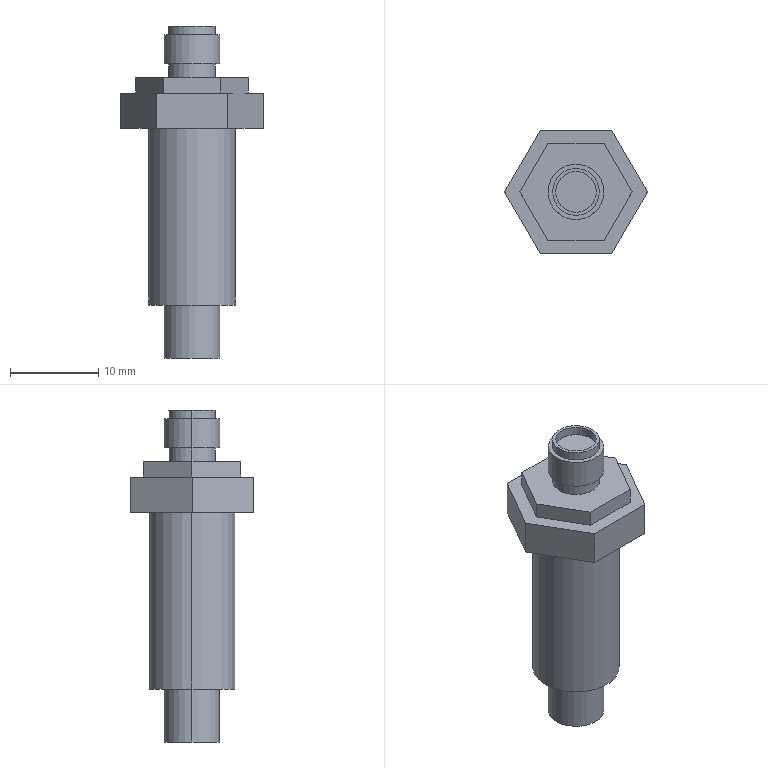Part | SolidWorks | features ICE 5, Extrusion 1 | 1 solid | 40 faces | box 16.166 x 14 x 37.6 mm | volume 2584 mm3 | plane 24 | cylinder 16 | commonest cylinder face diameters 4.6 x4 5.3 x4 6.3 x4 4.5 x2 9.8 x2
STEP:
#1=CARTESIAN_POINT('',(2.25,0.,-26.));
#2=VERTEX_POINT('',#1);
#3=CARTESIAN_POINT('',(-2.25,0.,-26.));
#4=VERTEX_POINT('',#3);
#5=CARTESIAN_POINT('',(0.,0.,-26.));
#6=DIRECTION('',(0.,0.,-1.));
#7=DIRECTION('',(-1.,0.,0.));
#8=AXIS2_PLACEMENT_3D('',#5,#6,#7);
#9=CIRCLE('',#8,2.25);
#10=EDGE_CURVE('',#2,#4,#9,.T.);
#11=ORIENTED_EDGE('',*,*,#10,.T.);
#12=CARTESIAN_POINT('',(-2.25,0.,-20.));
#13=VERTEX_POINT('',#12);
#14=CARTESIAN_POINT('',(-2.25,0.,-26.));
#15=DIRECTION('',(0.,0.,1.));
#16=VECTOR('',#15,1000.);
#17=LINE('',#14,#16);
#18=EDGE_CURVE('',#4,#13,#17,.T.);
#19=ORIENTED_EDGE('',*,*,#18,.T.);
#20=CARTESIAN_POINT('',(2.25,0.,-20.));
#21=VERTEX_POINT('',#20);
#22=CARTESIAN_POINT('',(0.,0.,-20.));
#23=DIRECTION('',(0.,0.,1.));
#24=DIRECTION('',(-1.,0.,0.));
#25=AXIS2_PLACEMENT_3D('',#22,#23,#24);
#26=CIRCLE('',#25,2.25);
#27=EDGE_CURVE('',#13,#21,#26,.T.);
#28=ORIENTED_EDGE('',*,*,#27,.T.);
#29=CARTESIAN_POINT('',(2.25,0.,-26.));
#30=DIRECTION('',(0.,0.,1.));
#31=VECTOR('',#30,1000.);
#32=LINE('',#29,#31);
#33=EDGE_CURVE('',#2,#21,#32,.T.);
#34=ORIENTED_EDGE('',*,*,#33,.F.);
#35=EDGE_LOOP('',(#11,#19,#28,#34));
#36=FACE_OUTER_BOUND('',#35,.T.);
#37=CARTESIAN_POINT('',(0.,0.,-26.));
#38=DIRECTION('',(0.,0.,1.));
#39=DIRECTION('',(1.,0.,0.));
#40=AXIS2_PLACEMENT_3D('',#37,#38,#39);
#41=CYLINDRICAL_SURFACE('',#40,2.25);
#42=ADVANCED_FACE('',(#36),#41,.F.);
#43=CARTESIAN_POINT('',(-3.15,0.,-26.));
#44=VERTEX_POINT('',#43);
#45=CARTESIAN_POINT('',(3.15,0.,-26.));
#46=VERTEX_POINT('',#45);
#47=CARTESIAN_POINT('',(0.,0.,-26.));
#48=DIRECTION('',(0.,0.,-1.));
#49=DIRECTION('',(-1.,0.,0.));
#50=AXIS2_PLACEMENT_3D('',#47,#48,#49);
#51=CIRCLE('',#50,3.15);
#52=EDGE_CURVE('',#44,#46,#51,.T.);
#53=ORIENTED_EDGE('',*,*,#52,.F.);
#54=CARTESIAN_POINT('',(-3.15,0.,-20.));
#55=VERTEX_POINT('',#54);
#56=CARTESIAN_POINT('',(-3.15,0.,-26.));
#57=DIRECTION('',(0.,0.,1.));
#58=VECTOR('',#57,1000.);
#59=LINE('',#56,#58);
#60=EDGE_CURVE('',#44,#55,#59,.T.);
#61=ORIENTED_EDGE('',*,*,#60,.T.);
#62=CARTESIAN_POINT('',(3.15,0.,-20.));
#63=VERTEX_POINT('',#62);
#64=CARTESIAN_POINT('',(0.,0.,-20.));
#65=DIRECTION('',(0.,0.,-1.));
#66=DIRECTION('',(-1.,0.,0.));
#67=AXIS2_PLACEMENT_3D('',#64,#65,#66);
#68=CIRCLE('',#67,3.15);
#69=EDGE_CURVE('',#55,#63,#68,.T.);
#70=ORIENTED_EDGE('',*,*,#69,.T.);
#71=CARTESIAN_POINT('',(3.15,0.,-26.));
#72=DIRECTION('',(0.,0.,1.));
#73=VECTOR('',#72,1000.);
#74=LINE('',#71,#73);
#75=EDGE_CURVE('',#46,#63,#74,.T.);
#76=ORIENTED_EDGE('',*,*,#75,.F.);
#77=EDGE_LOOP('',(#53,#61,#70,#76));
#78=FACE_OUTER_BOUND('',#77,.T.);
#79=CARTESIAN_POINT('',(0.,0.,-26.));
#80=DIRECTION('',(0.,0.,1.));
#81=DIRECTION('',(1.,0.,0.));
#82=AXIS2_PLACEMENT_3D('',#79,#80,#81);
#83=CYLINDRICAL_SURFACE('',#82,3.15);
#84=ADVANCED_FACE('',(#78),#83,.T.);
#85=CARTESIAN_POINT('',(-4.9,0.,-20.));
#86=VERTEX_POINT('',#85);
#87=CARTESIAN_POINT('',(4.9,0.,-20.));
#88=VERTEX_POINT('',#87);
#89=CARTESIAN_POINT('',(0.,0.,-20.));
#90=DIRECTION('',(0.,0.,-1.));
#91=DIRECTION('',(-1.,0.,0.));
#92=AXIS2_PLACEMENT_3D('',#89,#90,#91);
#93=CIRCLE('',#92,4.9);
#94=EDGE_CURVE('',#86,#88,#93,.T.);
#95=ORIENTED_EDGE('',*,*,#94,.F.);
#96=CARTESIAN_POINT('',(-4.9,0.,0.));
#97=VERTEX_POINT('',#96);
#98=CARTESIAN_POINT('',(-4.9,0.,-20.));
#99=DIRECTION('',(0.,0.,1.));
#100=VECTOR('',#99,1000.);
#101=LINE('',#98,#100);
#102=EDGE_CURVE('',#86,#97,#101,.T.);
#103=ORIENTED_EDGE('',*,*,#102,.T.);
#104=CARTESIAN_POINT('',(4.9,0.,0.));
#105=VERTEX_POINT('',#104);
#106=CARTESIAN_POINT('',(0.,0.,0.));
#107=DIRECTION('',(0.,0.,-1.));
#108=DIRECTION('',(-1.,0.,0.));
#109=AXIS2_PLACEMENT_3D('',#106,#107,#108);
#110=CIRCLE('',#109,4.9);
#111=EDGE_CURVE('',#97,#105,#110,.T.);
#112=ORIENTED_EDGE('',*,*,#111,.T.);
#113=CARTESIAN_POINT('',(4.9,0.,-20.));
#114=DIRECTION('',(0.,0.,1.));
#115=VECTOR('',#114,1000.);
#116=LINE('',#113,#115);
#117=EDGE_CURVE('',#88,#105,#116,.T.);
#118=ORIENTED_EDGE('',*,*,#117,.F.);
#119=EDGE_LOOP('',(#95,#103,#112,#118));
#120=FACE_OUTER_BOUND('',#119,.T.);
#121=CARTESIAN_POINT('',(0.,0.,-20.));
#122=DIRECTION('',(0.,0.,1.));
#123=DIRECTION('',(1.,0.,0.));
#124=AXIS2_PLACEMENT_3D('',#121,#122,#123);
#125=CYLINDRICAL_SURFACE('',#124,4.9);
#126=ADVANCED_FACE('',(#120),#125,.T.);
#127=CARTESIAN_POINT('',(-2.3,0.,11.6));
#128=VERTEX_POINT('',#127);
#129=CARTESIAN_POINT('',(2.3,0.,11.6));
#130=VERTEX_POINT('',#129);
#131=CARTESIAN_POINT('',(0.,0.,11.6));
#132=DIRECTION('',(0.,0.,1.));
#133=DIRECTION('',(1.,0.,0.));
#134=AXIS2_PLACEMENT_3D('',#131,#132,#133);
#135=CIRCLE('',#134,2.3);
#136=EDGE_CURVE('',#128,#130,#135,.T.);
#137=ORIENTED_EDGE('',*,*,#136,.T.);
#138=CARTESIAN_POINT('',(2.3,0.,10.6));
#139=VERTEX_POINT('',#138);
#140=CARTESIAN_POINT('',(2.3,0.,11.6));
#141=DIRECTION('',(0.,0.,-1.));
#142=VECTOR('',#141,1000.);
#143=LINE('',#140,#142);
#144=EDGE_CURVE('',#130,#139,#143,.T.);
#145=ORIENTED_EDGE('',*,*,#144,.T.);
#146=CARTESIAN_POINT('',(-2.3,0.,10.6));
#147=VERTEX_POINT('',#146);
#148=CARTESIAN_POINT('',(0.,0.,10.6));
#149=DIRECTION('',(0.,0.,1.));
#150=DIRECTION('',(1.,0.,0.));
#151=AXIS2_PLACEMENT_3D('',#148,#149,#150);
#152=CIRCLE('',#151,2.3);
#153=EDGE_CURVE('',#147,#139,#152,.T.);
#154=ORIENTED_EDGE('',*,*,#153,.F.);
#155=CARTESIAN_POINT('',(-2.3,0.,11.6));
#156=DIRECTION('',(0.,0.,-1.));
#157=VECTOR('',#156,1000.);
#158=LINE('',#155,#157);
#159=EDGE_CURVE('',#128,#147,#158,.T.);
#160=ORIENTED_EDGE('',*,*,#159,.F.);
#161=EDGE_LOOP('',(#137,#145,#154,#160));
#162=FACE_OUTER_BOUND('',#161,.T.);
#163=CARTESIAN_POINT('',(0.,0.,11.6));
#164=DIRECTION('',(0.,0.,-1.));
#165=DIRECTION('',(-1.,0.,0.));
#166=AXIS2_PLACEMENT_3D('',#163,#164,#165);
#167=CYLINDRICAL_SURFACE('',#166,2.3);
#168=ADVANCED_FACE('',(#162),#167,.F.);
#169=CARTESIAN_POINT('',(2.65,0.,11.6));
#170=VERTEX_POINT('',#169);
#171=CARTESIAN_POINT('',(-2.65,0.,11.6));
#172=VERTEX_POINT('',#171);
#173=CARTESIAN_POINT('',(0.,0.,11.6));
#174=DIRECTION('',(0.,0.,1.));
#175=DIRECTION('',(1.,0.,0.));
#176=AXIS2_PLACEMENT_3D('',#173,#174,#175);
#177=CIRCLE('',#176,2.65);
#178=EDGE_CURVE('',#170,#172,#177,.T.);
#179=ORIENTED_EDGE('',*,*,#178,.F.);
#180=CARTESIAN_POINT('',(2.65,0.,10.6));
#181=VERTEX_POINT('',#180);
#182=CARTESIAN_POINT('',(2.65,0.,11.6));
#183=DIRECTION('',(0.,0.,-1.));
#184=VECTOR('',#183,1000.);
#185=LINE('',#182,#184);
#186=EDGE_CURVE('',#170,#181,#185,.T.);
#187=ORIENTED_EDGE('',*,*,#186,.T.);
#188=CARTESIAN_POINT('',(-2.65,0.,10.6));
#189=VERTEX_POINT('',#188);
#190=CARTESIAN_POINT('',(0.,0.,10.6));
#191=DIRECTION('',(0.,0.,1.));
#192=DIRECTION('',(1.,0.,0.));
#193=AXIS2_PLACEMENT_3D('',#190,#191,#192);
#194=CIRCLE('',#193,2.65);
#195=EDGE_CURVE('',#181,#189,#194,.T.);
#196=ORIENTED_EDGE('',*,*,#195,.T.);
#197=CARTESIAN_POINT('',(-2.65,0.,11.6));
#198=DIRECTION('',(0.,0.,-1.));
#199=VECTOR('',#198,1000.);
#200=LINE('',#197,#199);
#201=EDGE_CURVE('',#172,#189,#200,.T.);
#202=ORIENTED_EDGE('',*,*,#201,.F.);
#203=EDGE_LOOP('',(#179,#187,#196,#202));
#204=FACE_OUTER_BOUND('',#203,.T.);
#205=CARTESIAN_POINT('',(0.,0.,11.6));
#206=DIRECTION('',(0.,0.,-1.));
#207=DIRECTION('',(-1.,0.,0.));
#208=AXIS2_PLACEMENT_3D('',#205,#206,#207);
#209=CYLINDRICAL_SURFACE('',#208,2.65);
#210=ADVANCED_FACE('',(#204),#209,.T.);
#211=CARTESIAN_POINT('',(3.15,0.,7.3));
#212=VERTEX_POINT('',#211);
#213=CARTESIAN_POINT('',(-3.15,0.,7.3));
#214=VERTEX_POINT('',#213);
#215=CARTESIAN_POINT('',(0.,0.,7.3));
#216=DIRECTION('',(0.,0.,1.));
#217=DIRECTION('',(1.,0.,0.));
#218=AXIS2_PLACEMENT_3D('',#215,#216,#217);
#219=CIRCLE('',#218,3.15);
#220=EDGE_CURVE('',#212,#214,#219,.T.);
#221=ORIENTED_EDGE('',*,*,#220,.T.);
#222=CARTESIAN_POINT('',(-3.15,0.,10.6));
#223=VERTEX_POINT('',#222);
#224=CARTESIAN_POINT('',(-3.15,0.,7.3));
#225=DIRECTION('',(0.,0.,1.));
#226=VECTOR('',#225,1000.);
#227=LINE('',#224,#226);
#228=EDGE_CURVE('',#214,#223,#227,.T.);
#229=ORIENTED_EDGE('',*,*,#228,.T.);
#230=CARTESIAN_POINT('',(3.15,0.,10.6));
#231=VERTEX_POINT('',#230);
#232=CARTESIAN_POINT('',(0.,0.,10.6));
#233=DIRECTION('',(0.,0.,1.));
#234=DIRECTION('',(1.,0.,0.));
#235=AXIS2_PLACEMENT_3D('',#232,#233,#234);
#236=CIRCLE('',#235,3.15);
#237=EDGE_CURVE('',#231,#223,#236,.T.);
#238=ORIENTED_EDGE('',*,*,#237,.F.);
#239=CARTESIAN_POINT('',(3.15,0.,7.3));
#240=DIRECTION('',(0.,0.,1.));
#241=VECTOR('',#240,1000.);
#242=LINE('',#239,#241);
#243=EDGE_CURVE('',#212,#231,#242,.T.);
#244=ORIENTED_EDGE('',*,*,#243,.F.);
#245=EDGE_LOOP('',(#221,#229,#238,#244));
#246=FACE_OUTER_BOUND('',#245,.T.);
#247=CARTESIAN_POINT('',(0.,0.,7.3));
#248=DIRECTION('',(0.,0.,1.));
#249=DIRECTION('',(1.,0.,0.));
#250=AXIS2_PLACEMENT_3D('',#247,#248,#249);
#251=CYLINDRICAL_SURFACE('',#250,3.15);
#252=ADVANCED_FACE('',(#246),#251,.T.);
#253=CARTESIAN_POINT('',(2.65,0.,7.3));
#254=VERTEX_POINT('',#253);
#255=CARTESIAN_POINT('',(-2.65,0.,7.3));
#256=VERTEX_POINT('',#255);
#257=CARTESIAN_POINT('',(0.,0.,7.3));
#258=DIRECTION('',(0.,0.,1.));
#259=DIRECTION('',(1.,0.,0.));
#260=AXIS2_PLACEMENT_3D('',#257,#258,#259);
#261=CIRCLE('',#260,2.65);
#262=EDGE_CURVE('',#254,#256,#261,.T.);
#263=ORIENTED_EDGE('',*,*,#262,.F.);
#264=CARTESIAN_POINT('',(2.65,0.,5.8));
#265=VERTEX_POINT('',#264);
#266=CARTESIAN_POINT('',(2.65,0.,11.6));
#267=DIRECTION('',(0.,0.,-1.));
#268=VECTOR('',#267,1000.);
#269=LINE('',#266,#268);
#270=EDGE_CURVE('',#254,#265,#269,.T.);
#271=ORIENTED_EDGE('',*,*,#270,.T.);
#272=CARTESIAN_POINT('',(-2.65,0.,5.8));
#273=VERTEX_POINT('',#272);
#274=CARTESIAN_POINT('',(0.,0.,5.8));
#275=DIRECTION('',(0.,0.,1.));
#276=DIRECTION('',(1.,0.,0.));
#277=AXIS2_PLACEMENT_3D('',#274,#275,#276);
#278=CIRCLE('',#277,2.65);
#279=EDGE_CURVE('',#265,#273,#278,.T.);
#280=ORIENTED_EDGE('',*,*,#279,.T.);
#281=CARTESIAN_POINT('',(-2.65,0.,11.6));
#282=DIRECTION('',(0.,0.,-1.));
#283=VECTOR('',#282,1000.);
#284=LINE('',#281,#283);
#285=EDGE_CURVE('',#256,#273,#284,.T.);
#286=ORIENTED_EDGE('',*,*,#285,.F.);
#287=EDGE_LOOP('',(#263,#271,#280,#286));
#288=FACE_OUTER_BOUND('',#287,.T.);
#289=CARTESIAN_POINT('',(0.,0.,11.6));
#290=DIRECTION('',(0.,0.,-1.));
#291=DIRECTION('',(-1.,0.,0.));
#292=AXIS2_PLACEMENT_3D('',#289,#290,#291);
#293=CYLINDRICAL_SURFACE('',#292,2.65);
#294=ADVANCED_FACE('',(#288),#293,.T.);
#295=ORIENTED_EDGE('',*,*,#270,.F.);
#296=CARTESIAN_POINT('',(0.,0.,7.3));
#297=DIRECTION('',(0.,0.,1.));
#298=DIRECTION('',(1.,0.,0.));
#299=AXIS2_PLACEMENT_3D('',#296,#297,#298);
#300=CIRCLE('',#299,2.65);
#301=EDGE_CURVE('',#256,#254,#300,.T.);
#302=ORIENTED_EDGE('',*,*,#301,.F.);
#303=ORIENTED_EDGE('',*,*,#285,.T.);
#304=CARTESIAN_POINT('',(0.,0.,5.8));
#305=DIRECTION('',(0.,0.,1.));
#306=DIRECTION('',(1.,0.,0.));
#307=AXIS2_PLACEMENT_3D('',#304,#305,#306);
#308=CIRCLE('',#307,2.65);
#309=EDGE_CURVE('',#273,#265,#308,.T.);
#310=ORIENTED_EDGE('',*,*,#309,.T.);
#311=EDGE_LOOP('',(#295,#302,#303,#310));
#312=FACE_OUTER_BOUND('',#311,.T.);
#313=CARTESIAN_POINT('',(0.,0.,11.6));
#314=DIRECTION('',(0.,0.,-1.));
#315=DIRECTION('',(-1.,0.,0.));
#316=AXIS2_PLACEMENT_3D('',#313,#314,#315);
#317=CYLINDRICAL_SURFACE('',#316,2.65);
#318=ADVANCED_FACE('',(#312),#317,.T.);
#319=CARTESIAN_POINT('',(4.041,-7.,0.));
#320=VERTEX_POINT('',#319);
#321=CARTESIAN_POINT('',(8.083,0.,0.));
#322=VERTEX_POINT('',#321);
#323=CARTESIAN_POINT('',(4.041,-7.,0.));
#324=DIRECTION('',(0.5,0.866,0.));
#325=VECTOR('',#324,1000.);
#326=LINE('',#323,#325);
#327=EDGE_CURVE('',#320,#322,#326,.T.);
#328=ORIENTED_EDGE('',*,*,#327,.T.);
#329=CARTESIAN_POINT('',(8.083,0.,4.));
#330=VERTEX_POINT('',#329);
#331=CARTESIAN_POINT('',(8.083,0.,4.));
#332=DIRECTION('',(0.,0.,-1.));
#333=VECTOR('',#332,1000.);
#334=LINE('',#331,#333);
#335=EDGE_CURVE('',#330,#322,#334,.T.);
#336=ORIENTED_EDGE('',*,*,#335,.F.);
#337=CARTESIAN_POINT('',(4.041,-7.,4.));
#338=VERTEX_POINT('',#337);
#339=CARTESIAN_POINT('',(4.041,-7.,4.));
#340=DIRECTION('',(0.5,0.866,0.));
#341=VECTOR('',#340,1000.);
#342=LINE('',#339,#341);
#343=EDGE_CURVE('',#338,#330,#342,.T.);
#344=ORIENTED_EDGE('',*,*,#343,.F.);
#345=CARTESIAN_POINT('',(4.041,-7.,4.));
#346=DIRECTION('',(0.,0.,-1.));
#347=VECTOR('',#346,1000.);
#348=LINE('',#345,#347);
#349=EDGE_CURVE('',#338,#320,#348,.T.);
#350=ORIENTED_EDGE('',*,*,#349,.T.);
#351=EDGE_LOOP('',(#328,#336,#344,#350));
#352=FACE_OUTER_BOUND('',#351,.T.);
#353=CARTESIAN_POINT('',(4.041,-7.,4.));
#354=DIRECTION('',(-0.866,0.5,0.));
#355=DIRECTION('',(-0.5,-0.866,0.));
#356=AXIS2_PLACEMENT_3D('',#353,#354,#355);
#357=PLANE('',#356);
#358=ADVANCED_FACE('',(#352),#357,.F.);
#359=CARTESIAN_POINT('',(4.041,7.,0.));
#360=VERTEX_POINT('',#359);
#361=CARTESIAN_POINT('',(8.083,0.,0.));
#362=DIRECTION('',(-0.5,0.866,0.));
#363=VECTOR('',#362,1000.);
#364=LINE('',#361,#363);
#365=EDGE_CURVE('',#322,#360,#364,.T.);
#366=ORIENTED_EDGE('',*,*,#365,.T.);
#367=CARTESIAN_POINT('',(4.041,7.,4.));
#368=VERTEX_POINT('',#367);
#369=CARTESIAN_POINT('',(4.041,7.,4.));
#370=DIRECTION('',(0.,0.,-1.));
#371=VECTOR('',#370,1000.);
#372=LINE('',#369,#371);
#373=EDGE_CURVE('',#368,#360,#372,.T.);
#374=ORIENTED_EDGE('',*,*,#373,.F.);
#375=CARTESIAN_POINT('',(8.083,0.,4.));
#376=DIRECTION('',(-0.5,0.866,0.));
#377=VECTOR('',#376,1000.);
#378=LINE('',#375,#377);
#379=EDGE_CURVE('',#330,#368,#378,.T.);
#380=ORIENTED_EDGE('',*,*,#379,.F.);
#381=ORIENTED_EDGE('',*,*,#335,.T.);
#382=EDGE_LOOP('',(#366,#374,#380,#381));
#383=FACE_OUTER_BOUND('',#382,.T.);
#384=CARTESIAN_POINT('',(8.083,0.,4.));
#385=DIRECTION('',(-0.866,-0.5,0.));
#386=DIRECTION('',(0.5,-0.866,0.));
#387=AXIS2_PLACEMENT_3D('',#384,#385,#386);
#388=PLANE('',#387);
#389=ADVANCED_FACE('',(#383),#388,.F.);
#390=CARTESIAN_POINT('',(-4.041,7.,0.));
#391=VERTEX_POINT('',#390);
#392=CARTESIAN_POINT('',(4.041,7.,0.));
#393=DIRECTION('',(-1.,0.,0.));
#394=VECTOR('',#393,1000.);
#395=LINE('',#392,#394);
#396=EDGE_CURVE('',#360,#391,#395,.T.);
#397=ORIENTED_EDGE('',*,*,#396,.T.);
#398=CARTESIAN_POINT('',(-4.041,7.,4.));
#399=VERTEX_POINT('',#398);
#400=CARTESIAN_POINT('',(-4.041,7.,4.));
#401=DIRECTION('',(0.,0.,-1.));
#402=VECTOR('',#401,1000.);
#403=LINE('',#400,#402);
#404=EDGE_CURVE('',#399,#391,#403,.T.);
#405=ORIENTED_EDGE('',*,*,#404,.F.);
#406=CARTESIAN_POINT('',(4.041,7.,4.));
#407=DIRECTION('',(-1.,0.,0.));
#408=VECTOR('',#407,1000.);
#409=LINE('',#406,#408);
#410=EDGE_CURVE('',#368,#399,#409,.T.);
#411=ORIENTED_EDGE('',*,*,#410,.F.);
#412=ORIENTED_EDGE('',*,*,#373,.T.);
#413=EDGE_LOOP('',(#397,#405,#411,#412));
#414=FACE_OUTER_BOUND('',#413,.T.);
#415=CARTESIAN_POINT('',(4.041,7.,4.));
#416=DIRECTION('',(0.,-1.,0.));
#417=DIRECTION('',(1.,0.,0.));
#418=AXIS2_PLACEMENT_3D('',#415,#416,#417);
#419=PLANE('',#418);
#420=ADVANCED_FACE('',(#414),#419,.F.);
#421=CARTESIAN_POINT('',(-8.083,0.,0.));
#422=VERTEX_POINT('',#421);
#423=CARTESIAN_POINT('',(-4.041,7.,0.));
#424=DIRECTION('',(-0.5,-0.866,0.));
#425=VECTOR('',#424,1000.);
#426=LINE('',#423,#425);
#427=EDGE_CURVE('',#391,#422,#426,.T.);
#428=ORIENTED_EDGE('',*,*,#427,.T.);
#429=CARTESIAN_POINT('',(-8.083,0.,4.));
#430=VERTEX_POINT('',#429);
#431=CARTESIAN_POINT('',(-8.083,0.,4.));
#432=DIRECTION('',(0.,0.,-1.));
#433=VECTOR('',#432,1000.);
#434=LINE('',#431,#433);
#435=EDGE_CURVE('',#430,#422,#434,.T.);
#436=ORIENTED_EDGE('',*,*,#435,.F.);
#437=CARTESIAN_POINT('',(-4.041,7.,4.));
#438=DIRECTION('',(-0.5,-0.866,0.));
#439=VECTOR('',#438,1000.);
#440=LINE('',#437,#439);
#441=EDGE_CURVE('',#399,#430,#440,.T.);
#442=ORIENTED_EDGE('',*,*,#441,.F.);
#443=ORIENTED_EDGE('',*,*,#404,.T.);
#444=EDGE_LOOP('',(#428,#436,#442,#443));
#445=FACE_OUTER_BOUND('',#444,.T.);
#446=CARTESIAN_POINT('',(-4.041,7.,4.));
#447=DIRECTION('',(0.866,-0.5,0.));
#448=DIRECTION('',(0.5,0.866,0.));
#449=AXIS2_PLACEMENT_3D('',#446,#447,#448);
#450=PLANE('',#449);
#451=ADVANCED_FACE('',(#445),#450,.F.);
#452=CARTESIAN_POINT('',(-4.041,-7.,0.));
#453=VERTEX_POINT('',#452);
#454=CARTESIAN_POINT('',(-8.083,0.,0.));
#455=DIRECTION('',(0.5,-0.866,0.));
#456=VECTOR('',#455,1000.);
#457=LINE('',#454,#456);
#458=EDGE_CURVE('',#422,#453,#457,.T.);
#459=ORIENTED_EDGE('',*,*,#458,.T.);
#460=CARTESIAN_POINT('',(-4.041,-7.,4.));
#461=VERTEX_POINT('',#460);
#462=CARTESIAN_POINT('',(-4.041,-7.,4.));
#463=DIRECTION('',(0.,0.,-1.));
#464=VECTOR('',#463,1000.);
#465=LINE('',#462,#464);
#466=EDGE_CURVE('',#461,#453,#465,.T.);
#467=ORIENTED_EDGE('',*,*,#466,.F.);
#468=CARTESIAN_POINT('',(-8.083,0.,4.));
#469=DIRECTION('',(0.5,-0.866,0.));
#470=VECTOR('',#469,1000.);
#471=LINE('',#468,#470);
#472=EDGE_CURVE('',#430,#461,#471,.T.);
#473=ORIENTED_EDGE('',*,*,#472,.F.);
#474=ORIENTED_EDGE('',*,*,#435,.T.);
#475=EDGE_LOOP('',(#459,#467,#473,#474));
#476=FACE_OUTER_BOUND('',#475,.T.);
#477=CARTESIAN_POINT('',(-8.083,0.,4.));
#478=DIRECTION('',(0.866,0.5,0.));
#479=DIRECTION('',(-0.5,0.866,0.));
#480=AXIS2_PLACEMENT_3D('',#477,#478,#479);
#481=PLANE('',#480);
#482=ADVANCED_FACE('',(#476),#481,.F.);
#483=CARTESIAN_POINT('',(-4.041,-7.,0.));
#484=DIRECTION('',(1.,0.,0.));
#485=VECTOR('',#484,1000.);
#486=LINE('',#483,#485);
#487=EDGE_CURVE('',#453,#320,#486,.T.);
#488=ORIENTED_EDGE('',*,*,#487,.T.);
#489=ORIENTED_EDGE('',*,*,#349,.F.);
#490=CARTESIAN_POINT('',(-4.041,-7.,4.));
#491=DIRECTION('',(1.,0.,0.));
#492=VECTOR('',#491,1000.);
#493=LINE('',#490,#492);
#494=EDGE_CURVE('',#461,#338,#493,.T.);
#495=ORIENTED_EDGE('',*,*,#494,.F.);
#496=ORIENTED_EDGE('',*,*,#466,.T.);
#497=EDGE_LOOP('',(#488,#489,#495,#496));
#498=FACE_OUTER_BOUND('',#497,.T.);
#499=CARTESIAN_POINT('',(-4.041,-7.,4.));
#500=DIRECTION('',(0.,1.,0.));
#501=DIRECTION('',(-1.,0.,0.));
#502=AXIS2_PLACEMENT_3D('',#499,#500,#501);
#503=PLANE('',#502);
#504=ADVANCED_FACE('',(#498),#503,.F.);
#505=CARTESIAN_POINT('',(3.175,-5.5,4.));
#506=VERTEX_POINT('',#505);
#507=CARTESIAN_POINT('',(6.351,0.,4.));
#508=VERTEX_POINT('',#507);
#509=CARTESIAN_POINT('',(3.175,-5.5,4.));
#510=DIRECTION('',(0.5,0.866,0.));
#511=VECTOR('',#510,1000.);
#512=LINE('',#509,#511);
#513=EDGE_CURVE('',#506,#508,#512,.T.);
#514=ORIENTED_EDGE('',*,*,#513,.F.);
#515=CARTESIAN_POINT('',(-3.175,-5.5,4.));
#516=VERTEX_POINT('',#515);
#517=CARTESIAN_POINT('',(-3.175,-5.5,4.));
#518=DIRECTION('',(1.,0.,0.));
#519=VECTOR('',#518,1000.);
#520=LINE('',#517,#519);
#521=EDGE_CURVE('',#516,#506,#520,.T.);
#522=ORIENTED_EDGE('',*,*,#521,.F.);
#523=CARTESIAN_POINT('',(-6.351,0.,4.));
#524=VERTEX_POINT('',#523);
#525=CARTESIAN_POINT('',(-6.351,0.,4.));
#526=DIRECTION('',(0.5,-0.866,0.));
#527=VECTOR('',#526,1000.);
#528=LINE('',#525,#527);
#529=EDGE_CURVE('',#524,#516,#528,.T.);
#530=ORIENTED_EDGE('',*,*,#529,.F.);
#531=CARTESIAN_POINT('',(-3.175,5.5,4.));
#532=VERTEX_POINT('',#531);
#533=CARTESIAN_POINT('',(-3.175,5.5,4.));
#534=DIRECTION('',(-0.5,-0.866,0.));
#535=VECTOR('',#534,1000.);
#536=LINE('',#533,#535);
#537=EDGE_CURVE('',#532,#524,#536,.T.);
#538=ORIENTED_EDGE('',*,*,#537,.F.);
#539=CARTESIAN_POINT('',(3.175,5.5,4.));
#540=VERTEX_POINT('',#539);
#541=CARTESIAN_POINT('',(3.175,5.5,4.));
#542=DIRECTION('',(-1.,0.,0.));
#543=VECTOR('',#542,1000.);
#544=LINE('',#541,#543);
#545=EDGE_CURVE('',#540,#532,#544,.T.);
#546=ORIENTED_EDGE('',*,*,#545,.F.);
#547=CARTESIAN_POINT('',(6.351,0.,4.));
#548=DIRECTION('',(-0.5,0.866,0.));
#549=VECTOR('',#548,1000.);
#550=LINE('',#547,#549);
#551=EDGE_CURVE('',#508,#540,#550,.T.);
#552=ORIENTED_EDGE('',*,*,#551,.F.);
#553=EDGE_LOOP('',(#514,#522,#530,#538,#546,#552));
#554=FACE_BOUND('',#553,.T.);
#555=ORIENTED_EDGE('',*,*,#343,.T.);
#556=ORIENTED_EDGE('',*,*,#379,.T.);
#557=ORIENTED_EDGE('',*,*,#410,.T.);
#558=ORIENTED_EDGE('',*,*,#441,.T.);
#559=ORIENTED_EDGE('',*,*,#472,.T.);
#560=ORIENTED_EDGE('',*,*,#494,.T.);
#561=EDGE_LOOP('',(#555,#556,#557,#558,#559,#560));
#562=FACE_OUTER_BOUND('',#561,.T.);
#563=CARTESIAN_POINT('',(0.,0.,4.));
#564=DIRECTION('',(0.,0.,1.));
#565=DIRECTION('',(1.,0.,0.));
#566=AXIS2_PLACEMENT_3D('',#563,#564,#565);
#567=PLANE('',#566);
#568=ADVANCED_FACE('',(#554,#562),#567,.T.);
#569=CARTESIAN_POINT('',(0.,0.,0.));
#570=DIRECTION('',(0.,0.,-1.));
#571=DIRECTION('',(-1.,0.,0.));
#572=AXIS2_PLACEMENT_3D('',#569,#570,#571);
#573=CIRCLE('',#572,4.9);
#574=EDGE_CURVE('',#105,#97,#573,.T.);
#575=ORIENTED_EDGE('',*,*,#574,.F.);
#576=ORIENTED_EDGE('',*,*,#111,.F.);
#577=EDGE_LOOP('',(#575,#576));
#578=FACE_BOUND('',#577,.T.);
#579=ORIENTED_EDGE('',*,*,#327,.F.);
#580=ORIENTED_EDGE('',*,*,#487,.F.);
#581=ORIENTED_EDGE('',*,*,#458,.F.);
#582=ORIENTED_EDGE('',*,*,#427,.F.);
#583=ORIENTED_EDGE('',*,*,#396,.F.);
#584=ORIENTED_EDGE('',*,*,#365,.F.);
#585=EDGE_LOOP('',(#579,#580,#581,#582,#583,#584));
#586=FACE_OUTER_BOUND('',#585,.T.);
#587=CARTESIAN_POINT('',(0.,0.,0.));
#588=DIRECTION('',(0.,0.,1.));
#589=DIRECTION('',(1.,0.,0.));
#590=AXIS2_PLACEMENT_3D('',#587,#588,#589);
#591=PLANE('',#590);
#592=ADVANCED_FACE('',(#578,#586),#591,.F.);
#593=ORIENTED_EDGE('',*,*,#513,.T.);
#594=CARTESIAN_POINT('',(6.351,0.,5.8));
#595=VERTEX_POINT('',#594);
#596=CARTESIAN_POINT('',(6.351,0.,5.8));
#597=DIRECTION('',(0.,0.,-1.));
#598=VECTOR('',#597,1000.);
#599=LINE('',#596,#598);
#600=EDGE_CURVE('',#595,#508,#599,.T.);
#601=ORIENTED_EDGE('',*,*,#600,.F.);
#602=CARTESIAN_POINT('',(3.175,-5.5,5.8));
#603=VERTEX_POINT('',#602);
#604=CARTESIAN_POINT('',(3.175,-5.5,5.8));
#605=DIRECTION('',(0.5,0.866,0.));
#606=VECTOR('',#605,1000.);
#607=LINE('',#604,#606);
#608=EDGE_CURVE('',#603,#595,#607,.T.);
#609=ORIENTED_EDGE('',*,*,#608,.F.);
#610=CARTESIAN_POINT('',(3.175,-5.5,5.8));
#611=DIRECTION('',(0.,0.,-1.));
#612=VECTOR('',#611,1000.);
#613=LINE('',#610,#612);
#614=EDGE_CURVE('',#603,#506,#613,.T.);
#615=ORIENTED_EDGE('',*,*,#614,.T.);
#616=EDGE_LOOP('',(#593,#601,#609,#615));
#617=FACE_OUTER_BOUND('',#616,.T.);
#618=CARTESIAN_POINT('',(3.175,-5.5,5.8));
#619=DIRECTION('',(-0.866,0.5,0.));
#620=DIRECTION('',(-0.5,-0.866,0.));
#621=AXIS2_PLACEMENT_3D('',#618,#619,#620);
#622=PLANE('',#621);
#623=ADVANCED_FACE('',(#617),#622,.F.);
#624=ORIENTED_EDGE('',*,*,#551,.T.);
#625=CARTESIAN_POINT('',(3.175,5.5,5.8));
#626=VERTEX_POINT('',#625);
#627=CARTESIAN_POINT('',(3.175,5.5,5.8));
#628=DIRECTION('',(0.,0.,-1.));
#629=VECTOR('',#628,1000.);
#630=LINE('',#627,#629);
#631=EDGE_CURVE('',#626,#540,#630,.T.);
#632=ORIENTED_EDGE('',*,*,#631,.F.);
#633=CARTESIAN_POINT('',(6.351,0.,5.8));
#634=DIRECTION('',(-0.5,0.866,0.));
#635=VECTOR('',#634,1000.);
#636=LINE('',#633,#635);
#637=EDGE_CURVE('',#595,#626,#636,.T.);
#638=ORIENTED_EDGE('',*,*,#637,.F.);
#639=ORIENTED_EDGE('',*,*,#600,.T.);
#640=EDGE_LOOP('',(#624,#632,#638,#639));
#641=FACE_OUTER_BOUND('',#640,.T.);
#642=CARTESIAN_POINT('',(6.351,0.,5.8));
#643=DIRECTION('',(-0.866,-0.5,0.));
#644=DIRECTION('',(0.5,-0.866,0.));
#645=AXIS2_PLACEMENT_3D('',#642,#643,#644);
#646=PLANE('',#645);
#647=ADVANCED_FACE('',(#641),#646,.F.);
#648=ORIENTED_EDGE('',*,*,#545,.T.);
#649=CARTESIAN_POINT('',(-3.175,5.5,5.8));
#650=VERTEX_POINT('',#649);
#651=CARTESIAN_POINT('',(-3.175,5.5,5.8));
#652=DIRECTION('',(0.,0.,-1.));
#653=VECTOR('',#652,1000.);
#654=LINE('',#651,#653);
#655=EDGE_CURVE('',#650,#532,#654,.T.);
#656=ORIENTED_EDGE('',*,*,#655,.F.);
#657=CARTESIAN_POINT('',(3.175,5.5,5.8));
#658=DIRECTION('',(-1.,0.,0.));
#659=VECTOR('',#658,1000.);
#660=LINE('',#657,#659);
#661=EDGE_CURVE('',#626,#650,#660,.T.);
#662=ORIENTED_EDGE('',*,*,#661,.F.);
#663=ORIENTED_EDGE('',*,*,#631,.T.);
#664=EDGE_LOOP('',(#648,#656,#662,#663));
#665=FACE_OUTER_BOUND('',#664,.T.);
#666=CARTESIAN_POINT('',(3.175,5.5,5.8));
#667=DIRECTION('',(0.,-1.,0.));
#668=DIRECTION('',(0.,0.,-1.));
#669=AXIS2_PLACEMENT_3D('',#666,#667,#668);
#670=PLANE('',#669);
#671=ADVANCED_FACE('',(#665),#670,.F.);
#672=ORIENTED_EDGE('',*,*,#537,.T.);
#673=CARTESIAN_POINT('',(-6.351,0.,5.8));
#674=VERTEX_POINT('',#673);
#675=CARTESIAN_POINT('',(-6.351,0.,5.8));
#676=DIRECTION('',(0.,0.,-1.));
#677=VECTOR('',#676,1000.);
#678=LINE('',#675,#677);
#679=EDGE_CURVE('',#674,#524,#678,.T.);
#680=ORIENTED_EDGE('',*,*,#679,.F.);
#681=CARTESIAN_POINT('',(-3.175,5.5,5.8));
#682=DIRECTION('',(-0.5,-0.866,0.));
#683=VECTOR('',#682,1000.);
#684=LINE('',#681,#683);
#685=EDGE_CURVE('',#650,#674,#684,.T.);
#686=ORIENTED_EDGE('',*,*,#685,.F.);
#687=ORIENTED_EDGE('',*,*,#655,.T.);
#688=EDGE_LOOP('',(#672,#680,#686,#687));
#689=FACE_OUTER_BOUND('',#688,.T.);
#690=CARTESIAN_POINT('',(-3.175,5.5,5.8));
#691=DIRECTION('',(0.866,-0.5,0.));
#692=DIRECTION('',(0.5,0.866,0.));
#693=AXIS2_PLACEMENT_3D('',#690,#691,#692);
#694=PLANE('',#693);
#695=ADVANCED_FACE('',(#689),#694,.F.);
#696=ORIENTED_EDGE('',*,*,#529,.T.);
#697=CARTESIAN_POINT('',(-3.175,-5.5,5.8));
#698=VERTEX_POINT('',#697);
#699=CARTESIAN_POINT('',(-3.175,-5.5,5.8));
#700=DIRECTION('',(0.,0.,-1.));
#701=VECTOR('',#700,1000.);
#702=LINE('',#699,#701);
#703=EDGE_CURVE('',#698,#516,#702,.T.);
#704=ORIENTED_EDGE('',*,*,#703,.F.);
#705=CARTESIAN_POINT('',(-6.351,0.,5.8));
#706=DIRECTION('',(0.5,-0.866,0.));
#707=VECTOR('',#706,1000.);
#708=LINE('',#705,#707);
#709=EDGE_CURVE('',#674,#698,#708,.T.);
#710=ORIENTED_EDGE('',*,*,#709,.F.);
#711=ORIENTED_EDGE('',*,*,#679,.T.);
#712=EDGE_LOOP('',(#696,#704,#710,#711));
#713=FACE_OUTER_BOUND('',#712,.T.);
#714=CARTESIAN_POINT('',(-6.351,0.,5.8));
#715=DIRECTION('',(0.866,0.5,0.));
#716=DIRECTION('',(-0.5,0.866,0.));
#717=AXIS2_PLACEMENT_3D('',#714,#715,#716);
#718=PLANE('',#717);
#719=ADVANCED_FACE('',(#713),#718,.F.);
#720=ORIENTED_EDGE('',*,*,#521,.T.);
#721=ORIENTED_EDGE('',*,*,#614,.F.);
#722=CARTESIAN_POINT('',(-3.175,-5.5,5.8));
#723=DIRECTION('',(1.,0.,0.));
#724=VECTOR('',#723,1000.);
#725=LINE('',#722,#724);
#726=EDGE_CURVE('',#698,#603,#725,.T.);
#727=ORIENTED_EDGE('',*,*,#726,.F.);
#728=ORIENTED_EDGE('',*,*,#703,.T.);
#729=EDGE_LOOP('',(#720,#721,#727,#728));
#730=FACE_OUTER_BOUND('',#729,.T.);
#731=CARTESIAN_POINT('',(-3.175,-5.5,5.8));
#732=DIRECTION('',(0.,1.,0.));
#733=DIRECTION('',(-1.,0.,0.));
#734=AXIS2_PLACEMENT_3D('',#731,#732,#733);
#735=PLANE('',#734);
#736=ADVANCED_FACE('',(#730),#735,.F.);
#737=ORIENTED_EDGE('',*,*,#309,.F.);
#738=ORIENTED_EDGE('',*,*,#279,.F.);
#739=EDGE_LOOP('',(#737,#738));
#740=FACE_BOUND('',#739,.T.);
#741=ORIENTED_EDGE('',*,*,#608,.T.);
#742=ORIENTED_EDGE('',*,*,#637,.T.);
#743=ORIENTED_EDGE('',*,*,#661,.T.);
#744=ORIENTED_EDGE('',*,*,#685,.T.);
#745=ORIENTED_EDGE('',*,*,#709,.T.);
#746=ORIENTED_EDGE('',*,*,#726,.T.);
#747=EDGE_LOOP('',(#741,#742,#743,#744,#745,#746));
#748=FACE_OUTER_BOUND('',#747,.T.);
#749=CARTESIAN_POINT('',(0.,0.,5.8));
#750=DIRECTION('',(0.,0.,1.));
#751=DIRECTION('',(1.,0.,0.));
#752=AXIS2_PLACEMENT_3D('',#749,#750,#751);
#753=PLANE('',#752);
#754=ADVANCED_FACE('',(#740,#748),#753,.T.);
#755=ORIENTED_EDGE('',*,*,#228,.F.);
#756=CARTESIAN_POINT('',(0.,0.,7.3));
#757=DIRECTION('',(0.,0.,1.));
#758=DIRECTION('',(1.,0.,0.));
#759=AXIS2_PLACEMENT_3D('',#756,#757,#758);
#760=CIRCLE('',#759,3.15);
#761=EDGE_CURVE('',#214,#212,#760,.T.);
#762=ORIENTED_EDGE('',*,*,#761,.T.);
#763=ORIENTED_EDGE('',*,*,#243,.T.);
#764=CARTESIAN_POINT('',(0.,0.,10.6));
#765=DIRECTION('',(0.,0.,1.));
#766=DIRECTION('',(1.,0.,0.));
#767=AXIS2_PLACEMENT_3D('',#764,#765,#766);
#768=CIRCLE('',#767,3.15);
#769=EDGE_CURVE('',#223,#231,#768,.T.);
#770=ORIENTED_EDGE('',*,*,#769,.F.);
#771=EDGE_LOOP('',(#755,#762,#763,#770));
#772=FACE_OUTER_BOUND('',#771,.T.);
#773=CARTESIAN_POINT('',(0.,0.,7.3));
#774=DIRECTION('',(0.,0.,1.));
#775=DIRECTION('',(1.,0.,0.));
#776=AXIS2_PLACEMENT_3D('',#773,#774,#775);
#777=CYLINDRICAL_SURFACE('',#776,3.15);
#778=ADVANCED_FACE('',(#772),#777,.T.);
#779=ORIENTED_EDGE('',*,*,#301,.T.);
#780=ORIENTED_EDGE('',*,*,#262,.T.);
#781=EDGE_LOOP('',(#779,#780));
#782=FACE_BOUND('',#781,.T.);
#783=ORIENTED_EDGE('',*,*,#220,.F.);
#784=ORIENTED_EDGE('',*,*,#761,.F.);
#785=EDGE_LOOP('',(#783,#784));
#786=FACE_OUTER_BOUND('',#785,.T.);
#787=CARTESIAN_POINT('',(0.,0.,7.3));
#788=DIRECTION('',(0.,0.,1.));
#789=DIRECTION('',(1.,0.,0.));
#790=AXIS2_PLACEMENT_3D('',#787,#788,#789);
#791=PLANE('',#790);
#792=ADVANCED_FACE('',(#782,#786),#791,.F.);
#793=CARTESIAN_POINT('',(0.,0.,10.6));
#794=DIRECTION('',(0.,0.,1.));
#795=DIRECTION('',(1.,0.,0.));
#796=AXIS2_PLACEMENT_3D('',#793,#794,#795);
#797=CIRCLE('',#796,2.65);
#798=EDGE_CURVE('',#189,#181,#797,.T.);
#799=ORIENTED_EDGE('',*,*,#798,.F.);
#800=ORIENTED_EDGE('',*,*,#195,.F.);
#801=EDGE_LOOP('',(#799,#800));
#802=FACE_BOUND('',#801,.T.);
#803=ORIENTED_EDGE('',*,*,#237,.T.);
#804=ORIENTED_EDGE('',*,*,#769,.T.);
#805=EDGE_LOOP('',(#803,#804));
#806=FACE_OUTER_BOUND('',#805,.T.);
#807=CARTESIAN_POINT('',(0.,0.,10.6));
#808=DIRECTION('',(0.,0.,1.));
#809=DIRECTION('',(1.,0.,0.));
#810=AXIS2_PLACEMENT_3D('',#807,#808,#809);
#811=PLANE('',#810);
#812=ADVANCED_FACE('',(#802,#806),#811,.T.);
#813=ORIENTED_EDGE('',*,*,#186,.F.);
#814=CARTESIAN_POINT('',(0.,0.,11.6));
#815=DIRECTION('',(0.,0.,1.));
#816=DIRECTION('',(1.,0.,0.));
#817=AXIS2_PLACEMENT_3D('',#814,#815,#816);
#818=CIRCLE('',#817,2.65);
#819=EDGE_CURVE('',#172,#170,#818,.T.);
#820=ORIENTED_EDGE('',*,*,#819,.F.);
#821=ORIENTED_EDGE('',*,*,#201,.T.);
#822=ORIENTED_EDGE('',*,*,#798,.T.);
#823=EDGE_LOOP('',(#813,#820,#821,#822));
#824=FACE_OUTER_BOUND('',#823,.T.);
#825=CARTESIAN_POINT('',(0.,0.,11.6));
#826=DIRECTION('',(0.,0.,-1.));
#827=DIRECTION('',(-1.,0.,0.));
#828=AXIS2_PLACEMENT_3D('',#825,#826,#827);
#829=CYLINDRICAL_SURFACE('',#828,2.65);
#830=ADVANCED_FACE('',(#824),#829,.T.);
#831=ORIENTED_EDGE('',*,*,#819,.T.);
#832=ORIENTED_EDGE('',*,*,#178,.T.);
#833=EDGE_LOOP('',(#831,#832));
#834=FACE_OUTER_BOUND('',#833,.T.);
#835=ORIENTED_EDGE('',*,*,#136,.F.);
#836=CARTESIAN_POINT('',(0.,0.,11.6));
#837=DIRECTION('',(0.,0.,1.));
#838=DIRECTION('',(1.,0.,0.));
#839=AXIS2_PLACEMENT_3D('',#836,#837,#838);
#840=CIRCLE('',#839,2.3);
#841=EDGE_CURVE('',#130,#128,#840,.T.);
#842=ORIENTED_EDGE('',*,*,#841,.F.);
#843=EDGE_LOOP('',(#835,#842));
#844=FACE_BOUND('',#843,.T.);
#845=CARTESIAN_POINT('',(0.,0.,11.6));
#846=DIRECTION('',(0.,0.,1.));
#847=DIRECTION('',(1.,0.,0.));
#848=AXIS2_PLACEMENT_3D('',#845,#846,#847);
#849=PLANE('',#848);
#850=ADVANCED_FACE('',(#834,#844),#849,.T.);
#851=ORIENTED_EDGE('',*,*,#144,.F.);
#852=ORIENTED_EDGE('',*,*,#841,.T.);
#853=ORIENTED_EDGE('',*,*,#159,.T.);
#854=CARTESIAN_POINT('',(0.,0.,10.6));
#855=DIRECTION('',(0.,0.,1.));
#856=DIRECTION('',(1.,0.,0.));
#857=AXIS2_PLACEMENT_3D('',#854,#855,#856);
#858=CIRCLE('',#857,2.3);
#859=EDGE_CURVE('',#139,#147,#858,.T.);
#860=ORIENTED_EDGE('',*,*,#859,.F.);
#861=EDGE_LOOP('',(#851,#852,#853,#860));
#862=FACE_OUTER_BOUND('',#861,.T.);
#863=CARTESIAN_POINT('',(0.,0.,11.6));
#864=DIRECTION('',(0.,0.,-1.));
#865=DIRECTION('',(-1.,0.,0.));
#866=AXIS2_PLACEMENT_3D('',#863,#864,#865);
#867=CYLINDRICAL_SURFACE('',#866,2.3);
#868=ADVANCED_FACE('',(#862),#867,.F.);
#869=ORIENTED_EDGE('',*,*,#153,.T.);
#870=ORIENTED_EDGE('',*,*,#859,.T.);
#871=EDGE_LOOP('',(#869,#870));
#872=FACE_OUTER_BOUND('',#871,.T.);
#873=CARTESIAN_POINT('',(0.,0.,10.6));
#874=DIRECTION('',(0.,0.,1.));
#875=DIRECTION('',(1.,0.,0.));
#876=AXIS2_PLACEMENT_3D('',#873,#874,#875);
#877=PLANE('',#876);
#878=ADVANCED_FACE('',(#872),#877,.T.);
#879=ORIENTED_EDGE('',*,*,#102,.F.);
#880=CARTESIAN_POINT('',(0.,0.,-20.));
#881=DIRECTION('',(0.,0.,-1.));
#882=DIRECTION('',(-1.,0.,0.));
#883=AXIS2_PLACEMENT_3D('',#880,#881,#882);
#884=CIRCLE('',#883,4.9);
#885=EDGE_CURVE('',#88,#86,#884,.T.);
#886=ORIENTED_EDGE('',*,*,#885,.F.);
#887=ORIENTED_EDGE('',*,*,#117,.T.);
#888=ORIENTED_EDGE('',*,*,#574,.T.);
#889=EDGE_LOOP('',(#879,#886,#887,#888));
#890=FACE_OUTER_BOUND('',#889,.T.);
#891=CARTESIAN_POINT('',(0.,0.,-20.));
#892=DIRECTION('',(0.,0.,1.));
#893=DIRECTION('',(1.,0.,0.));
#894=AXIS2_PLACEMENT_3D('',#891,#892,#893);
#895=CYLINDRICAL_SURFACE('',#894,4.9);
#896=ADVANCED_FACE('',(#890),#895,.T.);
#897=CARTESIAN_POINT('',(0.,0.,-20.));
#898=DIRECTION('',(0.,0.,-1.));
#899=DIRECTION('',(-1.,0.,0.));
#900=AXIS2_PLACEMENT_3D('',#897,#898,#899);
#901=CIRCLE('',#900,3.15);
#902=EDGE_CURVE('',#63,#55,#901,.T.);
#903=ORIENTED_EDGE('',*,*,#902,.F.);
#904=ORIENTED_EDGE('',*,*,#69,.F.);
#905=EDGE_LOOP('',(#903,#904));
#906=FACE_BOUND('',#905,.T.);
#907=ORIENTED_EDGE('',*,*,#885,.T.);
#908=ORIENTED_EDGE('',*,*,#94,.T.);
#909=EDGE_LOOP('',(#907,#908));
#910=FACE_OUTER_BOUND('',#909,.T.);
#911=CARTESIAN_POINT('',(0.,0.,-20.));
#912=DIRECTION('',(0.,0.,-1.));
#913=DIRECTION('',(-1.,0.,0.));
#914=AXIS2_PLACEMENT_3D('',#911,#912,#913);
#915=PLANE('',#914);
#916=ADVANCED_FACE('',(#906,#910),#915,.T.);
#917=CARTESIAN_POINT('',(0.,0.,-26.));
#918=DIRECTION('',(0.,0.,-1.));
#919=DIRECTION('',(-1.,0.,0.));
#920=AXIS2_PLACEMENT_3D('',#917,#918,#919);
#921=CIRCLE('',#920,3.15);
#922=EDGE_CURVE('',#46,#44,#921,.T.);
#923=ORIENTED_EDGE('',*,*,#922,.T.);
#924=ORIENTED_EDGE('',*,*,#52,.T.);
#925=EDGE_LOOP('',(#923,#924));
#926=FACE_OUTER_BOUND('',#925,.T.);
#927=ORIENTED_EDGE('',*,*,#10,.F.);
#928=CARTESIAN_POINT('',(0.,0.,-26.));
#929=DIRECTION('',(0.,0.,-1.));
#930=DIRECTION('',(-1.,0.,0.));
#931=AXIS2_PLACEMENT_3D('',#928,#929,#930);
#932=CIRCLE('',#931,2.25);
#933=EDGE_CURVE('',#4,#2,#932,.T.);
#934=ORIENTED_EDGE('',*,*,#933,.F.);
#935=EDGE_LOOP('',(#927,#934));
#936=FACE_BOUND('',#935,.T.);
#937=CARTESIAN_POINT('',(0.,0.,-26.));
#938=DIRECTION('',(0.,0.,-1.));
#939=DIRECTION('',(-1.,0.,0.));
#940=AXIS2_PLACEMENT_3D('',#937,#938,#939);
#941=PLANE('',#940);
#942=ADVANCED_FACE('',(#926,#936),#941,.T.);
#943=ORIENTED_EDGE('',*,*,#60,.F.);
#944=ORIENTED_EDGE('',*,*,#922,.F.);
#945=ORIENTED_EDGE('',*,*,#75,.T.);
#946=ORIENTED_EDGE('',*,*,#902,.T.);
#947=EDGE_LOOP('',(#943,#944,#945,#946));
#948=FACE_OUTER_BOUND('',#947,.T.);
#949=CARTESIAN_POINT('',(0.,0.,-26.));
#950=DIRECTION('',(0.,0.,1.));
#951=DIRECTION('',(1.,0.,0.));
#952=AXIS2_PLACEMENT_3D('',#949,#950,#951);
#953=CYLINDRICAL_SURFACE('',#952,3.15);
#954=ADVANCED_FACE('',(#948),#953,.T.);
#955=ORIENTED_EDGE('',*,*,#18,.F.);
#956=ORIENTED_EDGE('',*,*,#933,.T.);
#957=ORIENTED_EDGE('',*,*,#33,.T.);
#958=CARTESIAN_POINT('',(0.,0.,-20.));
#959=DIRECTION('',(0.,0.,1.));
#960=DIRECTION('',(-1.,0.,0.));
#961=AXIS2_PLACEMENT_3D('',#958,#959,#960);
#962=CIRCLE('',#961,2.25);
#963=EDGE_CURVE('',#21,#13,#962,.T.);
#964=ORIENTED_EDGE('',*,*,#963,.T.);
#965=EDGE_LOOP('',(#955,#956,#957,#964));
#966=FACE_OUTER_BOUND('',#965,.T.);
#967=CARTESIAN_POINT('',(0.,0.,-26.));
#968=DIRECTION('',(0.,0.,1.));
#969=DIRECTION('',(1.,0.,0.));
#970=AXIS2_PLACEMENT_3D('',#967,#968,#969);
#971=CYLINDRICAL_SURFACE('',#970,2.25);
#972=ADVANCED_FACE('',(#966),#971,.F.);
#973=ORIENTED_EDGE('',*,*,#963,.F.);
#974=ORIENTED_EDGE('',*,*,#27,.F.);
#975=EDGE_LOOP('',(#973,#974));
#976=FACE_OUTER_BOUND('',#975,.T.);
#977=CARTESIAN_POINT('',(0.,0.,-20.));
#978=DIRECTION('',(0.,0.,-1.));
#979=DIRECTION('',(-1.,0.,0.));
#980=AXIS2_PLACEMENT_3D('',#977,#978,#979);
#981=PLANE('',#980);
#982=ADVANCED_FACE('',(#976),#981,.T.);
#983=CLOSED_SHELL('',(#42,#84,#126,#168,#210,#252,#294,#318,#358,#389,#420,#451,#482,#504,#568,#592,#623,#647,#671,#695,#719,#736,#754,#778,#792,#812,#830,#850,#868,#878,#896,#916,#942,#954,#972,#982));
#984=CARTESIAN_POINT('',(-2.3,0.,7.3));
#985=VERTEX_POINT('',#984);
#986=CARTESIAN_POINT('',(2.3,0.,7.3));
#987=VERTEX_POINT('',#986);
#988=CARTESIAN_POINT('',(0.,0.,7.3));
#989=DIRECTION('',(0.,0.,1.));
#990=DIRECTION('',(1.,0.,0.));
#991=AXIS2_PLACEMENT_3D('',#988,#989,#990);
#992=CIRCLE('',#991,2.3);
#993=EDGE_CURVE('',#985,#987,#992,.T.);
#994=ORIENTED_EDGE('',*,*,#993,.T.);
#995=CARTESIAN_POINT('',(2.3,0.,5.8));
#996=VERTEX_POINT('',#995);
#997=CARTESIAN_POINT('',(2.3,0.,11.6));
#998=DIRECTION('',(0.,0.,-1.));
#999=VECTOR('',#998,1000.);
#1000=LINE('',#997,#999);
#1001=EDGE_CURVE('',#987,#996,#1000,.T.);
#1002=ORIENTED_EDGE('',*,*,#1001,.T.);
#1003=CARTESIAN_POINT('',(-2.3,0.,5.8));
#1004=VERTEX_POINT('',#1003);
#1005=CARTESIAN_POINT('',(0.,0.,5.8));
#1006=DIRECTION('',(0.,0.,-1.));
#1007=DIRECTION('',(1.,0.,0.));
#1008=AXIS2_PLACEMENT_3D('',#1005,#1006,#1007);
#1009=CIRCLE('',#1008,2.3);
#1010=EDGE_CURVE('',#996,#1004,#1009,.T.);
#1011=ORIENTED_EDGE('',*,*,#1010,.T.);
#1012=CARTESIAN_POINT('',(-2.3,0.,11.6));
#1013=DIRECTION('',(0.,0.,-1.));
#1014=VECTOR('',#1013,1000.);
#1015=LINE('',#1012,#1014);
#1016=EDGE_CURVE('',#985,#1004,#1015,.T.);
#1017=ORIENTED_EDGE('',*,*,#1016,.F.);
#1018=EDGE_LOOP('',(#994,#1002,#1011,#1017));
#1019=FACE_OUTER_BOUND('',#1018,.T.);
#1020=CARTESIAN_POINT('',(0.,0.,11.6));
#1021=DIRECTION('',(0.,0.,-1.));
#1022=DIRECTION('',(-1.,0.,0.));
#1023=AXIS2_PLACEMENT_3D('',#1020,#1021,#1022);
#1024=CYLINDRICAL_SURFACE('',#1023,2.3);
#1025=ADVANCED_FACE('',(#1019),#1024,.F.);
#1026=CARTESIAN_POINT('',(0.,0.,5.8));
#1027=DIRECTION('',(0.,0.,-1.));
#1028=DIRECTION('',(1.,0.,0.));
#1029=AXIS2_PLACEMENT_3D('',#1026,#1027,#1028);
#1030=CIRCLE('',#1029,2.3);
#1031=EDGE_CURVE('',#1004,#996,#1030,.T.);
#1032=ORIENTED_EDGE('',*,*,#1031,.F.);
#1033=ORIENTED_EDGE('',*,*,#1010,.F.);
#1034=EDGE_LOOP('',(#1032,#1033));
#1035=FACE_OUTER_BOUND('',#1034,.T.);
#1036=CARTESIAN_POINT('',(0.,0.,5.8));
#1037=DIRECTION('',(0.,0.,1.));
#1038=DIRECTION('',(1.,0.,0.));
#1039=AXIS2_PLACEMENT_3D('',#1036,#1037,#1038);
#1040=PLANE('',#1039);
#1041=ADVANCED_FACE('',(#1035),#1040,.T.);
#1042=ORIENTED_EDGE('',*,*,#1001,.F.);
#1043=CARTESIAN_POINT('',(0.,0.,7.3));
#1044=DIRECTION('',(0.,0.,1.));
#1045=DIRECTION('',(1.,0.,0.));
#1046=AXIS2_PLACEMENT_3D('',#1043,#1044,#1045);
#1047=CIRCLE('',#1046,2.3);
#1048=EDGE_CURVE('',#987,#985,#1047,.T.);
#1049=ORIENTED_EDGE('',*,*,#1048,.T.);
#1050=ORIENTED_EDGE('',*,*,#1016,.T.);
#1051=ORIENTED_EDGE('',*,*,#1031,.T.);
#1052=EDGE_LOOP('',(#1042,#1049,#1050,#1051));
#1053=FACE_OUTER_BOUND('',#1052,.T.);
#1054=CARTESIAN_POINT('',(0.,0.,11.6));
#1055=DIRECTION('',(0.,0.,-1.));
#1056=DIRECTION('',(-1.,0.,0.));
#1057=AXIS2_PLACEMENT_3D('',#1054,#1055,#1056);
#1058=CYLINDRICAL_SURFACE('',#1057,2.3);
#1059=ADVANCED_FACE('',(#1053),#1058,.F.);
#1060=ORIENTED_EDGE('',*,*,#993,.F.);
#1061=ORIENTED_EDGE('',*,*,#1048,.F.);
#1062=EDGE_LOOP('',(#1060,#1061));
#1063=FACE_OUTER_BOUND('',#1062,.T.);
#1064=CARTESIAN_POINT('',(0.,0.,7.3));
#1065=DIRECTION('',(0.,0.,1.));
#1066=DIRECTION('',(1.,0.,0.));
#1067=AXIS2_PLACEMENT_3D('',#1064,#1065,#1066);
#1068=PLANE('',#1067);
#1069=ADVANCED_FACE('',(#1063),#1068,.F.);
#1070=CLOSED_SHELL('',(#1025,#1041,#1059,#1069));
#1071=ORIENTED_CLOSED_SHELL('',*,#1070,.F.);
#1072=BREP_WITH_VOIDS('',#983,(#1071));
#1073=CARTESIAN_POINT('',(0.,0.,0.));
#1074=DIRECTION('',(0.,0.,1.));
#1075=DIRECTION('',(1.,0.,0.));
#1076=AXIS2_PLACEMENT_3D('',#1073,#1074,#1075);
#1077=(LENGTH_UNIT()NAMED_UNIT(*)SI_UNIT(.MILLI.,.METRE.));
#1078=UNCERTAINTY_MEASURE_WITH_UNIT(LENGTH_MEASURE(0.00001),#1077,'','');
#1079=(NAMED_UNIT(*)PLANE_ANGLE_UNIT()SI_UNIT($,.RADIAN.));
#1080=(NAMED_UNIT(*)SI_UNIT($,.STERADIAN.)SOLID_ANGLE_UNIT());
#1081=(GEOMETRIC_REPRESENTATION_CONTEXT(3)GLOBAL_UNCERTAINTY_ASSIGNED_CONTEXT((#1078))GLOBAL_UNIT_ASSIGNED_CONTEXT((#1077,#1079,#1080))REPRESENTATION_CONTEXT('',''));
#1082=ADVANCED_BREP_SHAPE_REPRESENTATION('',(#1072,#1076),#1081);